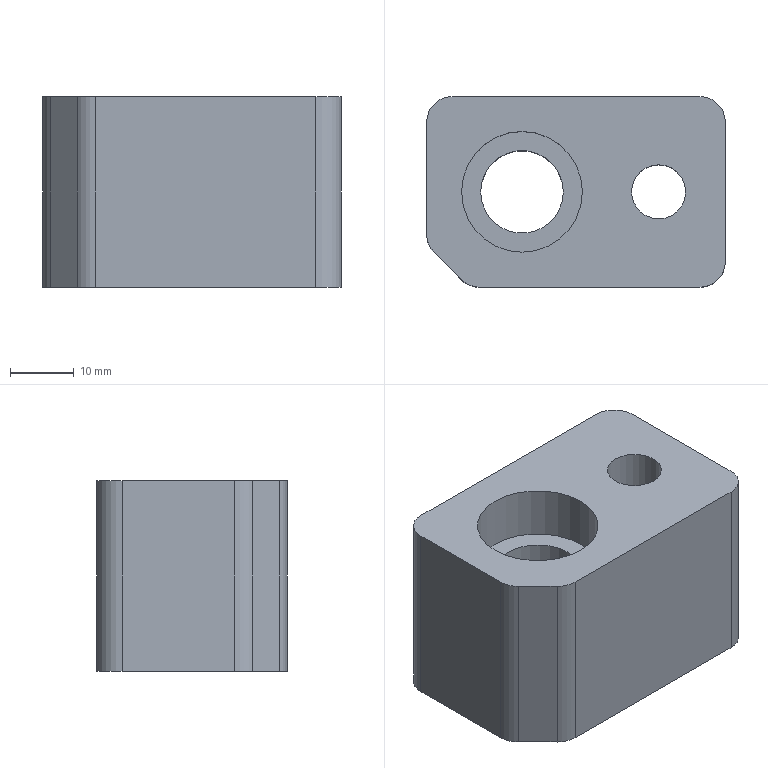Part | NX | features 7 2 | 1 solid | 18 faces | box 47 x 30 x 30 mm | volume 32748 mm3 | plane 9 | cylinder 9 | commonest cylinder face diameters 8 x5 8.5 x1 13 x1 14.5 x1 19 x1
STEP:
#1=CARTESIAN_POINT('',(3207.938,37.688,91.));
#2=VERTEX_POINT('',#1);
#3=CARTESIAN_POINT('',(3207.938,41.938,91.));
#4=DIRECTION('',(0.,0.,-1.));
#5=DIRECTION('',(0.,-1.,0.));
#6=AXIS2_PLACEMENT_3D('',#3,#4,#5);
#7=CIRCLE('',#6,4.25);
#8=EDGE_CURVE('',#2,#2,#7,.T.);
#9=ORIENTED_EDGE('',*,*,#8,.T.);
#10=EDGE_LOOP('',(#9));
#11=FACE_BOUND('',#10,.T.);
#12=CARTESIAN_POINT('',(3175.438,56.938,91.));
#13=VERTEX_POINT('',#12);
#14=CARTESIAN_POINT('',(3214.438,56.938,91.));
#15=VERTEX_POINT('',#14);
#16=CARTESIAN_POINT('',(3186.438,56.938,91.));
#17=DIRECTION('',(1.,0.,0.));
#18=VECTOR('',#17,1000.);
#19=LINE('',#16,#18);
#20=EDGE_CURVE('',#13,#15,#19,.T.);
#21=ORIENTED_EDGE('',*,*,#20,.F.);
#22=CARTESIAN_POINT('',(3171.438,52.938,91.));
#23=VERTEX_POINT('',#22);
#24=CARTESIAN_POINT('',(3175.438,52.938,91.));
#25=DIRECTION('',(0.,0.,1.));
#26=DIRECTION('',(0.,-1.,0.));
#27=AXIS2_PLACEMENT_3D('',#24,#25,#26);
#28=CIRCLE('',#27,4.);
#29=EDGE_CURVE('',#13,#23,#28,.T.);
#30=ORIENTED_EDGE('',*,*,#29,.T.);
#31=CARTESIAN_POINT('',(3171.438,35.231,91.));
#32=VERTEX_POINT('',#31);
#33=CARTESIAN_POINT('',(3171.438,41.938,91.));
#34=DIRECTION('',(0.,1.,0.));
#35=VECTOR('',#34,1000.);
#36=LINE('',#33,#35);
#37=EDGE_CURVE('',#32,#23,#36,.T.);
#38=ORIENTED_EDGE('',*,*,#37,.F.);
#39=CARTESIAN_POINT('',(3172.609,32.403,91.));
#40=VERTEX_POINT('',#39);
#41=CARTESIAN_POINT('',(3175.438,35.231,91.));
#42=DIRECTION('',(0.,0.,1.));
#43=DIRECTION('',(0.,-1.,0.));
#44=AXIS2_PLACEMENT_3D('',#41,#42,#43);
#45=CIRCLE('',#44,4.);
#46=EDGE_CURVE('',#32,#40,#45,.T.);
#47=ORIENTED_EDGE('',*,*,#46,.T.);
#48=CARTESIAN_POINT('',(3176.902,28.11,91.));
#49=VERTEX_POINT('',#48);
#50=CARTESIAN_POINT('',(3176.006,29.006,91.));
#51=DIRECTION('',(0.7071,-0.7071,0.));
#52=VECTOR('',#51,1000.);
#53=LINE('',#50,#52);
#54=EDGE_CURVE('',#40,#49,#53,.T.);
#55=ORIENTED_EDGE('',*,*,#54,.T.);
#56=CARTESIAN_POINT('',(3179.731,26.938,91.));
#57=VERTEX_POINT('',#56);
#58=CARTESIAN_POINT('',(3179.731,30.938,91.));
#59=DIRECTION('',(0.,0.,1.));
#60=DIRECTION('',(0.,-1.,0.));
#61=AXIS2_PLACEMENT_3D('',#58,#59,#60);
#62=CIRCLE('',#61,4.);
#63=EDGE_CURVE('',#49,#57,#62,.T.);
#64=ORIENTED_EDGE('',*,*,#63,.T.);
#65=CARTESIAN_POINT('',(3214.438,26.938,91.));
#66=VERTEX_POINT('',#65);
#67=CARTESIAN_POINT('',(3186.438,26.938,91.));
#68=DIRECTION('',(-1.,0.,0.));
#69=VECTOR('',#68,1000.);
#70=LINE('',#67,#69);
#71=EDGE_CURVE('',#66,#57,#70,.T.);
#72=ORIENTED_EDGE('',*,*,#71,.F.);
#73=CARTESIAN_POINT('',(3218.438,30.938,91.));
#74=VERTEX_POINT('',#73);
#75=CARTESIAN_POINT('',(3214.438,30.938,91.));
#76=DIRECTION('',(0.,0.,1.));
#77=DIRECTION('',(0.,-1.,0.));
#78=AXIS2_PLACEMENT_3D('',#75,#76,#77);
#79=CIRCLE('',#78,4.);
#80=EDGE_CURVE('',#66,#74,#79,.T.);
#81=ORIENTED_EDGE('',*,*,#80,.T.);
#82=CARTESIAN_POINT('',(3218.438,52.938,91.));
#83=VERTEX_POINT('',#82);
#84=CARTESIAN_POINT('',(3218.438,41.938,91.));
#85=DIRECTION('',(0.,-1.,0.));
#86=VECTOR('',#85,1000.);
#87=LINE('',#84,#86);
#88=EDGE_CURVE('',#83,#74,#87,.T.);
#89=ORIENTED_EDGE('',*,*,#88,.F.);
#90=CARTESIAN_POINT('',(3214.438,52.938,91.));
#91=DIRECTION('',(0.,0.,1.));
#92=DIRECTION('',(0.,-1.,0.));
#93=AXIS2_PLACEMENT_3D('',#90,#91,#92);
#94=CIRCLE('',#93,4.);
#95=EDGE_CURVE('',#83,#15,#94,.T.);
#96=ORIENTED_EDGE('',*,*,#95,.T.);
#97=EDGE_LOOP('',(#21,#30,#38,#47,#55,#64,#72,#81,#89,#96));
#98=FACE_BOUND('',#97,.T.);
#99=CARTESIAN_POINT('',(3195.938,41.938,91.));
#100=VERTEX_POINT('',#99);
#101=CARTESIAN_POINT('',(3186.438,41.938,91.));
#102=DIRECTION('',(0.,0.,-1.));
#103=DIRECTION('',(1.,0.,0.));
#104=AXIS2_PLACEMENT_3D('',#101,#102,#103);
#105=CIRCLE('',#104,9.5);
#106=EDGE_CURVE('',#100,#100,#105,.T.);
#107=ORIENTED_EDGE('',*,*,#106,.T.);
#108=EDGE_LOOP('',(#107));
#109=FACE_BOUND('',#108,.T.);
#110=CARTESIAN_POINT('',(3188.938,41.938,91.));
#111=DIRECTION('',(0.,0.,1.));
#112=DIRECTION('',(0.,1.,0.));
#113=AXIS2_PLACEMENT_3D('',#110,#111,#112);
#114=PLANE('',#113);
#115=ADVANCED_FACE('',(#11,#98,#109),#114,.T.);
#116=CARTESIAN_POINT('',(3179.938,41.938,61.));
#117=VERTEX_POINT('',#116);
#118=CARTESIAN_POINT('',(3186.438,41.938,61.));
#119=DIRECTION('',(0.,0.,-1.));
#120=DIRECTION('',(-1.,0.,0.));
#121=AXIS2_PLACEMENT_3D('',#118,#119,#120);
#122=CIRCLE('',#121,6.5);
#123=EDGE_CURVE('',#117,#117,#122,.T.);
#124=ORIENTED_EDGE('',*,*,#123,.F.);
#125=EDGE_LOOP('',(#124));
#126=FACE_BOUND('',#125,.T.);
#127=CARTESIAN_POINT('',(3207.938,49.188,61.));
#128=VERTEX_POINT('',#127);
#129=CARTESIAN_POINT('',(3207.938,41.938,61.));
#130=DIRECTION('',(0.,0.,-1.));
#131=DIRECTION('',(0.,1.,0.));
#132=AXIS2_PLACEMENT_3D('',#129,#130,#131);
#133=CIRCLE('',#132,7.25);
#134=EDGE_CURVE('',#128,#128,#133,.T.);
#135=ORIENTED_EDGE('',*,*,#134,.F.);
#136=EDGE_LOOP('',(#135));
#137=FACE_BOUND('',#136,.T.);
#138=CARTESIAN_POINT('',(3218.438,30.938,61.));
#139=VERTEX_POINT('',#138);
#140=CARTESIAN_POINT('',(3218.438,52.938,61.));
#141=VERTEX_POINT('',#140);
#142=CARTESIAN_POINT('',(3218.438,41.938,61.));
#143=DIRECTION('',(0.,1.,0.));
#144=VECTOR('',#143,1000.);
#145=LINE('',#142,#144);
#146=EDGE_CURVE('',#139,#141,#145,.T.);
#147=ORIENTED_EDGE('',*,*,#146,.F.);
#148=CARTESIAN_POINT('',(3214.438,26.938,61.));
#149=VERTEX_POINT('',#148);
#150=CARTESIAN_POINT('',(3214.438,30.938,61.));
#151=DIRECTION('',(0.,0.,-1.));
#152=DIRECTION('',(0.,1.,0.));
#153=AXIS2_PLACEMENT_3D('',#150,#151,#152);
#154=CIRCLE('',#153,4.);
#155=EDGE_CURVE('',#139,#149,#154,.T.);
#156=ORIENTED_EDGE('',*,*,#155,.T.);
#157=CARTESIAN_POINT('',(3179.731,26.938,61.));
#158=VERTEX_POINT('',#157);
#159=CARTESIAN_POINT('',(3186.438,26.938,61.));
#160=DIRECTION('',(1.,0.,0.));
#161=VECTOR('',#160,1000.);
#162=LINE('',#159,#161);
#163=EDGE_CURVE('',#158,#149,#162,.T.);
#164=ORIENTED_EDGE('',*,*,#163,.F.);
#165=CARTESIAN_POINT('',(3176.902,28.11,61.));
#166=VERTEX_POINT('',#165);
#167=CARTESIAN_POINT('',(3179.731,30.938,61.));
#168=DIRECTION('',(0.,0.,-1.));
#169=DIRECTION('',(0.,1.,0.));
#170=AXIS2_PLACEMENT_3D('',#167,#168,#169);
#171=CIRCLE('',#170,4.);
#172=EDGE_CURVE('',#158,#166,#171,.T.);
#173=ORIENTED_EDGE('',*,*,#172,.T.);
#174=CARTESIAN_POINT('',(3172.609,32.403,61.));
#175=VERTEX_POINT('',#174);
#176=CARTESIAN_POINT('',(3178.756,26.256,61.));
#177=DIRECTION('',(-0.7071,0.7071,0.));
#178=VECTOR('',#177,1000.);
#179=LINE('',#176,#178);
#180=EDGE_CURVE('',#166,#175,#179,.T.);
#181=ORIENTED_EDGE('',*,*,#180,.T.);
#182=CARTESIAN_POINT('',(3171.438,35.231,61.));
#183=VERTEX_POINT('',#182);
#184=CARTESIAN_POINT('',(3175.438,35.231,61.));
#185=DIRECTION('',(0.,0.,-1.));
#186=DIRECTION('',(0.,1.,0.));
#187=AXIS2_PLACEMENT_3D('',#184,#185,#186);
#188=CIRCLE('',#187,4.);
#189=EDGE_CURVE('',#175,#183,#188,.T.);
#190=ORIENTED_EDGE('',*,*,#189,.T.);
#191=CARTESIAN_POINT('',(3171.438,52.938,61.));
#192=VERTEX_POINT('',#191);
#193=CARTESIAN_POINT('',(3171.438,41.938,61.));
#194=DIRECTION('',(0.,-1.,0.));
#195=VECTOR('',#194,1000.);
#196=LINE('',#193,#195);
#197=EDGE_CURVE('',#192,#183,#196,.T.);
#198=ORIENTED_EDGE('',*,*,#197,.F.);
#199=CARTESIAN_POINT('',(3175.438,56.938,61.));
#200=VERTEX_POINT('',#199);
#201=CARTESIAN_POINT('',(3175.438,52.938,61.));
#202=DIRECTION('',(0.,0.,-1.));
#203=DIRECTION('',(0.,1.,0.));
#204=AXIS2_PLACEMENT_3D('',#201,#202,#203);
#205=CIRCLE('',#204,4.);
#206=EDGE_CURVE('',#192,#200,#205,.T.);
#207=ORIENTED_EDGE('',*,*,#206,.T.);
#208=CARTESIAN_POINT('',(3214.438,56.938,61.));
#209=VERTEX_POINT('',#208);
#210=CARTESIAN_POINT('',(3186.438,56.938,61.));
#211=DIRECTION('',(-1.,0.,0.));
#212=VECTOR('',#211,1000.);
#213=LINE('',#210,#212);
#214=EDGE_CURVE('',#209,#200,#213,.T.);
#215=ORIENTED_EDGE('',*,*,#214,.F.);
#216=CARTESIAN_POINT('',(3214.438,52.938,61.));
#217=DIRECTION('',(0.,0.,-1.));
#218=DIRECTION('',(0.,1.,0.));
#219=AXIS2_PLACEMENT_3D('',#216,#217,#218);
#220=CIRCLE('',#219,4.);
#221=EDGE_CURVE('',#209,#141,#220,.T.);
#222=ORIENTED_EDGE('',*,*,#221,.T.);
#223=EDGE_LOOP('',(#147,#156,#164,#173,#181,#190,#198,#207,#215,#222));
#224=FACE_BOUND('',#223,.T.);
#225=CARTESIAN_POINT('',(3371.438,218.938,61.));
#226=DIRECTION('',(0.,0.,-1.));
#227=DIRECTION('',(0.,-1.,0.));
#228=AXIS2_PLACEMENT_3D('',#225,#226,#227);
#229=PLANE('',#228);
#230=ADVANCED_FACE('',(#126,#137,#224),#229,.T.);
#231=ORIENTED_EDGE('',*,*,#37,.T.);
#232=CARTESIAN_POINT('',(3171.438,52.938,-5.));
#233=DIRECTION('',(0.,0.,-1.));
#234=VECTOR('',#233,1000.);
#235=LINE('',#232,#234);
#236=EDGE_CURVE('',#23,#192,#235,.T.);
#237=ORIENTED_EDGE('',*,*,#236,.T.);
#238=ORIENTED_EDGE('',*,*,#197,.T.);
#239=CARTESIAN_POINT('',(3171.438,35.231,-5.));
#240=DIRECTION('',(0.,0.,1.));
#241=VECTOR('',#240,1000.);
#242=LINE('',#239,#241);
#243=EDGE_CURVE('',#183,#32,#242,.T.);
#244=ORIENTED_EDGE('',*,*,#243,.T.);
#245=EDGE_LOOP('',(#231,#237,#238,#244));
#246=FACE_BOUND('',#245,.T.);
#247=CARTESIAN_POINT('',(3171.438,41.938,-5.));
#248=DIRECTION('',(-1.,0.,0.));
#249=DIRECTION('',(0.,0.,-1.));
#250=AXIS2_PLACEMENT_3D('',#247,#248,#249);
#251=PLANE('',#250);
#252=ADVANCED_FACE('',(#246),#251,.T.);
#253=ORIENTED_EDGE('',*,*,#71,.T.);
#254=CARTESIAN_POINT('',(3179.731,26.938,-5.));
#255=DIRECTION('',(0.,0.,-1.));
#256=VECTOR('',#255,1000.);
#257=LINE('',#254,#256);
#258=EDGE_CURVE('',#57,#158,#257,.T.);
#259=ORIENTED_EDGE('',*,*,#258,.T.);
#260=ORIENTED_EDGE('',*,*,#163,.T.);
#261=CARTESIAN_POINT('',(3214.438,26.938,-5.));
#262=DIRECTION('',(0.,0.,1.));
#263=VECTOR('',#262,1000.);
#264=LINE('',#261,#263);
#265=EDGE_CURVE('',#149,#66,#264,.T.);
#266=ORIENTED_EDGE('',*,*,#265,.T.);
#267=EDGE_LOOP('',(#253,#259,#260,#266));
#268=FACE_BOUND('',#267,.T.);
#269=CARTESIAN_POINT('',(3186.438,26.938,-5.));
#270=DIRECTION('',(0.,-1.,0.));
#271=DIRECTION('',(0.,0.,1.));
#272=AXIS2_PLACEMENT_3D('',#269,#270,#271);
#273=PLANE('',#272);
#274=ADVANCED_FACE('',(#268),#273,.T.);
#275=ORIENTED_EDGE('',*,*,#88,.T.);
#276=CARTESIAN_POINT('',(3218.438,30.938,-5.));
#277=DIRECTION('',(0.,0.,-1.));
#278=VECTOR('',#277,1000.);
#279=LINE('',#276,#278);
#280=EDGE_CURVE('',#74,#139,#279,.T.);
#281=ORIENTED_EDGE('',*,*,#280,.T.);
#282=ORIENTED_EDGE('',*,*,#146,.T.);
#283=CARTESIAN_POINT('',(3218.438,52.938,-5.));
#284=DIRECTION('',(0.,0.,1.));
#285=VECTOR('',#284,1000.);
#286=LINE('',#283,#285);
#287=EDGE_CURVE('',#141,#83,#286,.T.);
#288=ORIENTED_EDGE('',*,*,#287,.T.);
#289=EDGE_LOOP('',(#275,#281,#282,#288));
#290=FACE_BOUND('',#289,.T.);
#291=CARTESIAN_POINT('',(3218.438,41.938,-5.));
#292=DIRECTION('',(1.,0.,0.));
#293=DIRECTION('',(0.,0.,1.));
#294=AXIS2_PLACEMENT_3D('',#291,#292,#293);
#295=PLANE('',#294);
#296=ADVANCED_FACE('',(#290),#295,.T.);
#297=ORIENTED_EDGE('',*,*,#214,.T.);
#298=CARTESIAN_POINT('',(3175.438,56.938,-5.));
#299=DIRECTION('',(0.,0.,1.));
#300=VECTOR('',#299,1000.);
#301=LINE('',#298,#300);
#302=EDGE_CURVE('',#200,#13,#301,.T.);
#303=ORIENTED_EDGE('',*,*,#302,.T.);
#304=ORIENTED_EDGE('',*,*,#20,.T.);
#305=CARTESIAN_POINT('',(3214.438,56.938,-5.));
#306=DIRECTION('',(0.,0.,-1.));
#307=VECTOR('',#306,1000.);
#308=LINE('',#305,#307);
#309=EDGE_CURVE('',#15,#209,#308,.T.);
#310=ORIENTED_EDGE('',*,*,#309,.T.);
#311=EDGE_LOOP('',(#297,#303,#304,#310));
#312=FACE_BOUND('',#311,.T.);
#313=CARTESIAN_POINT('',(3186.438,56.938,-5.));
#314=DIRECTION('',(0.,1.,0.));
#315=DIRECTION('',(0.,0.,-1.));
#316=AXIS2_PLACEMENT_3D('',#313,#314,#315);
#317=PLANE('',#316);
#318=ADVANCED_FACE('',(#312),#317,.T.);
#319=ORIENTED_EDGE('',*,*,#54,.F.);
#320=CARTESIAN_POINT('',(3172.609,32.403,-5.));
#321=DIRECTION('',(0.,0.,-1.));
#322=VECTOR('',#321,1000.);
#323=LINE('',#320,#322);
#324=EDGE_CURVE('',#40,#175,#323,.T.);
#325=ORIENTED_EDGE('',*,*,#324,.T.);
#326=ORIENTED_EDGE('',*,*,#180,.F.);
#327=CARTESIAN_POINT('',(3176.902,28.11,-5.));
#328=DIRECTION('',(0.,0.,1.));
#329=VECTOR('',#328,1000.);
#330=LINE('',#327,#329);
#331=EDGE_CURVE('',#166,#49,#330,.T.);
#332=ORIENTED_EDGE('',*,*,#331,.T.);
#333=EDGE_LOOP('',(#319,#325,#326,#332));
#334=FACE_BOUND('',#333,.T.);
#335=CARTESIAN_POINT('',(3178.756,26.256,-5.));
#336=DIRECTION('',(0.7071,0.7071,0.));
#337=DIRECTION('',(0.,0.,1.));
#338=AXIS2_PLACEMENT_3D('',#335,#336,#337);
#339=PLANE('',#338);
#340=ADVANCED_FACE('',(#334),#339,.F.);
#341=ORIENTED_EDGE('',*,*,#221,.F.);
#342=ORIENTED_EDGE('',*,*,#309,.F.);
#343=ORIENTED_EDGE('',*,*,#95,.F.);
#344=ORIENTED_EDGE('',*,*,#287,.F.);
#345=EDGE_LOOP('',(#341,#342,#343,#344));
#346=FACE_BOUND('',#345,.T.);
#347=CARTESIAN_POINT('',(3214.438,52.938,-5.));
#348=DIRECTION('',(0.,0.,-1.));
#349=DIRECTION('',(0.,1.,0.));
#350=AXIS2_PLACEMENT_3D('',#347,#348,#349);
#351=CYLINDRICAL_SURFACE('',#350,4.);
#352=ADVANCED_FACE('',(#346),#351,.T.);
#353=ORIENTED_EDGE('',*,*,#155,.F.);
#354=ORIENTED_EDGE('',*,*,#280,.F.);
#355=ORIENTED_EDGE('',*,*,#80,.F.);
#356=ORIENTED_EDGE('',*,*,#265,.F.);
#357=EDGE_LOOP('',(#353,#354,#355,#356));
#358=FACE_BOUND('',#357,.T.);
#359=CARTESIAN_POINT('',(3214.438,30.938,-5.));
#360=DIRECTION('',(0.,0.,-1.));
#361=DIRECTION('',(0.,1.,0.));
#362=AXIS2_PLACEMENT_3D('',#359,#360,#361);
#363=CYLINDRICAL_SURFACE('',#362,4.);
#364=ADVANCED_FACE('',(#358),#363,.T.);
#365=ORIENTED_EDGE('',*,*,#172,.F.);
#366=ORIENTED_EDGE('',*,*,#258,.F.);
#367=ORIENTED_EDGE('',*,*,#63,.F.);
#368=ORIENTED_EDGE('',*,*,#331,.F.);
#369=EDGE_LOOP('',(#365,#366,#367,#368));
#370=FACE_BOUND('',#369,.T.);
#371=CARTESIAN_POINT('',(3179.731,30.938,-5.));
#372=DIRECTION('',(0.,0.,1.));
#373=DIRECTION('',(0.,-1.,0.));
#374=AXIS2_PLACEMENT_3D('',#371,#372,#373);
#375=CYLINDRICAL_SURFACE('',#374,4.);
#376=ADVANCED_FACE('',(#370),#375,.T.);
#377=ORIENTED_EDGE('',*,*,#46,.F.);
#378=ORIENTED_EDGE('',*,*,#243,.F.);
#379=ORIENTED_EDGE('',*,*,#189,.F.);
#380=ORIENTED_EDGE('',*,*,#324,.F.);
#381=EDGE_LOOP('',(#377,#378,#379,#380));
#382=FACE_BOUND('',#381,.T.);
#383=CARTESIAN_POINT('',(3175.438,35.231,-5.));
#384=DIRECTION('',(0.,0.,-1.));
#385=DIRECTION('',(0.,1.,0.));
#386=AXIS2_PLACEMENT_3D('',#383,#384,#385);
#387=CYLINDRICAL_SURFACE('',#386,4.);
#388=ADVANCED_FACE('',(#382),#387,.T.);
#389=ORIENTED_EDGE('',*,*,#206,.F.);
#390=ORIENTED_EDGE('',*,*,#236,.F.);
#391=ORIENTED_EDGE('',*,*,#29,.F.);
#392=ORIENTED_EDGE('',*,*,#302,.F.);
#393=EDGE_LOOP('',(#389,#390,#391,#392));
#394=FACE_BOUND('',#393,.T.);
#395=CARTESIAN_POINT('',(3175.438,52.938,-5.));
#396=DIRECTION('',(0.,0.,-1.));
#397=DIRECTION('',(0.,1.,0.));
#398=AXIS2_PLACEMENT_3D('',#395,#396,#397);
#399=CYLINDRICAL_SURFACE('',#398,4.);
#400=ADVANCED_FACE('',(#394),#399,.T.);
#401=CARTESIAN_POINT('',(3207.938,37.688,76.));
#402=VERTEX_POINT('',#401);
#403=CARTESIAN_POINT('',(3207.938,41.938,76.));
#404=DIRECTION('',(0.,0.,1.));
#405=DIRECTION('',(0.,-1.,0.));
#406=AXIS2_PLACEMENT_3D('',#403,#404,#405);
#407=CIRCLE('',#406,4.25);
#408=EDGE_CURVE('',#402,#402,#407,.T.);
#409=ORIENTED_EDGE('',*,*,#408,.F.);
#410=EDGE_LOOP('',(#409));
#411=FACE_BOUND('',#410,.T.);
#412=ORIENTED_EDGE('',*,*,#8,.F.);
#413=EDGE_LOOP('',(#412));
#414=FACE_BOUND('',#413,.T.);
#415=CARTESIAN_POINT('',(3207.938,41.938,55.));
#416=DIRECTION('',(0.,0.,1.));
#417=DIRECTION('',(0.,1.,0.));
#418=AXIS2_PLACEMENT_3D('',#415,#416,#417);
#419=CYLINDRICAL_SURFACE('',#418,4.25);
#420=ADVANCED_FACE('',(#411,#414),#419,.F.);
#421=ORIENTED_EDGE('',*,*,#408,.T.);
#422=EDGE_LOOP('',(#421));
#423=FACE_BOUND('',#422,.T.);
#424=CARTESIAN_POINT('',(3207.938,34.688,76.));
#425=VERTEX_POINT('',#424);
#426=CARTESIAN_POINT('',(3207.938,41.938,76.));
#427=DIRECTION('',(0.,0.,1.));
#428=DIRECTION('',(0.,-1.,0.));
#429=AXIS2_PLACEMENT_3D('',#426,#427,#428);
#430=CIRCLE('',#429,7.25);
#431=EDGE_CURVE('',#425,#425,#430,.T.);
#432=ORIENTED_EDGE('',*,*,#431,.F.);
#433=EDGE_LOOP('',(#432));
#434=FACE_BOUND('',#433,.T.);
#435=CARTESIAN_POINT('',(3207.938,41.938,76.));
#436=DIRECTION('',(0.,0.,1.));
#437=DIRECTION('',(0.,1.,0.));
#438=AXIS2_PLACEMENT_3D('',#435,#436,#437);
#439=PLANE('',#438);
#440=ADVANCED_FACE('',(#423,#434),#439,.F.);
#441=ORIENTED_EDGE('',*,*,#134,.T.);
#442=EDGE_LOOP('',(#441));
#443=FACE_BOUND('',#442,.T.);
#444=ORIENTED_EDGE('',*,*,#431,.T.);
#445=EDGE_LOOP('',(#444));
#446=FACE_BOUND('',#445,.T.);
#447=CARTESIAN_POINT('',(3207.938,41.938,55.));
#448=DIRECTION('',(0.,0.,1.));
#449=DIRECTION('',(0.,1.,0.));
#450=AXIS2_PLACEMENT_3D('',#447,#448,#449);
#451=CYLINDRICAL_SURFACE('',#450,7.25);
#452=ADVANCED_FACE('',(#443,#446),#451,.F.);
#453=CARTESIAN_POINT('',(3176.938,41.938,82.7));
#454=VERTEX_POINT('',#453);
#455=CARTESIAN_POINT('',(3186.438,41.938,82.7));
#456=DIRECTION('',(0.,0.,-1.));
#457=DIRECTION('',(-1.,0.,0.));
#458=AXIS2_PLACEMENT_3D('',#455,#456,#457);
#459=CIRCLE('',#458,9.5);
#460=EDGE_CURVE('',#454,#454,#459,.T.);
#461=ORIENTED_EDGE('',*,*,#460,.T.);
#462=EDGE_LOOP('',(#461));
#463=FACE_BOUND('',#462,.T.);
#464=ORIENTED_EDGE('',*,*,#106,.F.);
#465=EDGE_LOOP('',(#464));
#466=FACE_BOUND('',#465,.T.);
#467=CARTESIAN_POINT('',(3186.438,41.938,87.));
#468=DIRECTION('',(0.,0.,-1.));
#469=DIRECTION('',(-1.,0.,0.));
#470=AXIS2_PLACEMENT_3D('',#467,#468,#469);
#471=CYLINDRICAL_SURFACE('',#470,9.5);
#472=ADVANCED_FACE('',(#463,#466),#471,.F.);
#473=ORIENTED_EDGE('',*,*,#123,.T.);
#474=EDGE_LOOP('',(#473));
#475=FACE_BOUND('',#474,.T.);
#476=CARTESIAN_POINT('',(3179.938,41.938,82.7));
#477=VERTEX_POINT('',#476);
#478=CARTESIAN_POINT('',(3186.438,41.938,82.7));
#479=DIRECTION('',(0.,0.,-1.));
#480=DIRECTION('',(-1.,0.,0.));
#481=AXIS2_PLACEMENT_3D('',#478,#479,#480);
#482=CIRCLE('',#481,6.5);
#483=EDGE_CURVE('',#477,#477,#482,.T.);
#484=ORIENTED_EDGE('',*,*,#483,.F.);
#485=EDGE_LOOP('',(#484));
#486=FACE_BOUND('',#485,.T.);
#487=CARTESIAN_POINT('',(3186.438,41.938,46.5));
#488=DIRECTION('',(0.,0.,-1.));
#489=DIRECTION('',(-1.,0.,0.));
#490=AXIS2_PLACEMENT_3D('',#487,#488,#489);
#491=CYLINDRICAL_SURFACE('',#490,6.5);
#492=ADVANCED_FACE('',(#475,#486),#491,.F.);
#493=ORIENTED_EDGE('',*,*,#483,.T.);
#494=EDGE_LOOP('',(#493));
#495=FACE_BOUND('',#494,.T.);
#496=ORIENTED_EDGE('',*,*,#460,.F.);
#497=EDGE_LOOP('',(#496));
#498=FACE_BOUND('',#497,.T.);
#499=CARTESIAN_POINT('',(3186.438,41.938,82.7));
#500=DIRECTION('',(0.,0.,-1.));
#501=DIRECTION('',(0.,1.,0.));
#502=AXIS2_PLACEMENT_3D('',#499,#500,#501);
#503=PLANE('',#502);
#504=ADVANCED_FACE('',(#495,#498),#503,.F.);
#505=CLOSED_SHELL('',(#115,#230,#252,#274,#296,#318,#340,#352,#364,#376,#388,#400,#420,#440,#452,#472,#492,#504));
#506=MANIFOLD_SOLID_BREP('',#505);
#507=(LENGTH_UNIT()NAMED_UNIT(*)SI_UNIT(.MILLI.,.METRE.));
#508=UNCERTAINTY_MEASURE_WITH_UNIT(LENGTH_MEASURE(0.00001),#507,'','');
#509=(NAMED_UNIT(*)PLANE_ANGLE_UNIT()SI_UNIT($,.RADIAN.));
#510=(NAMED_UNIT(*)SI_UNIT($,.STERADIAN.)SOLID_ANGLE_UNIT());
#511=(GEOMETRIC_REPRESENTATION_CONTEXT(3)GLOBAL_UNCERTAINTY_ASSIGNED_CONTEXT((#508))GLOBAL_UNIT_ASSIGNED_CONTEXT((#507,#509,#510))REPRESENTATION_CONTEXT('',''));
#512=ADVANCED_BREP_SHAPE_REPRESENTATION('',(#506),#511);